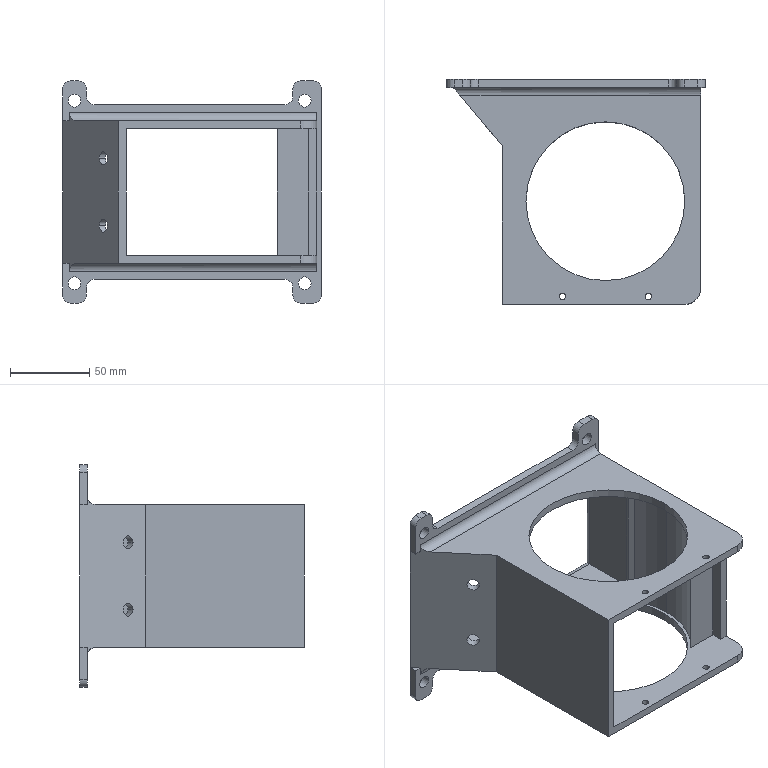Part | SolidWorks | features ICE 8, Fillet 6, Extrusion 1, Shell 1 | 1 solid | 79 faces | box 163 x 141.711 x 140 mm | volume 274719 mm3 | cylinder 47 | plane 32 | commonest cylinder face diameters 10 x19 8 x12 4 x8 100 x4 20 x2 104 x2